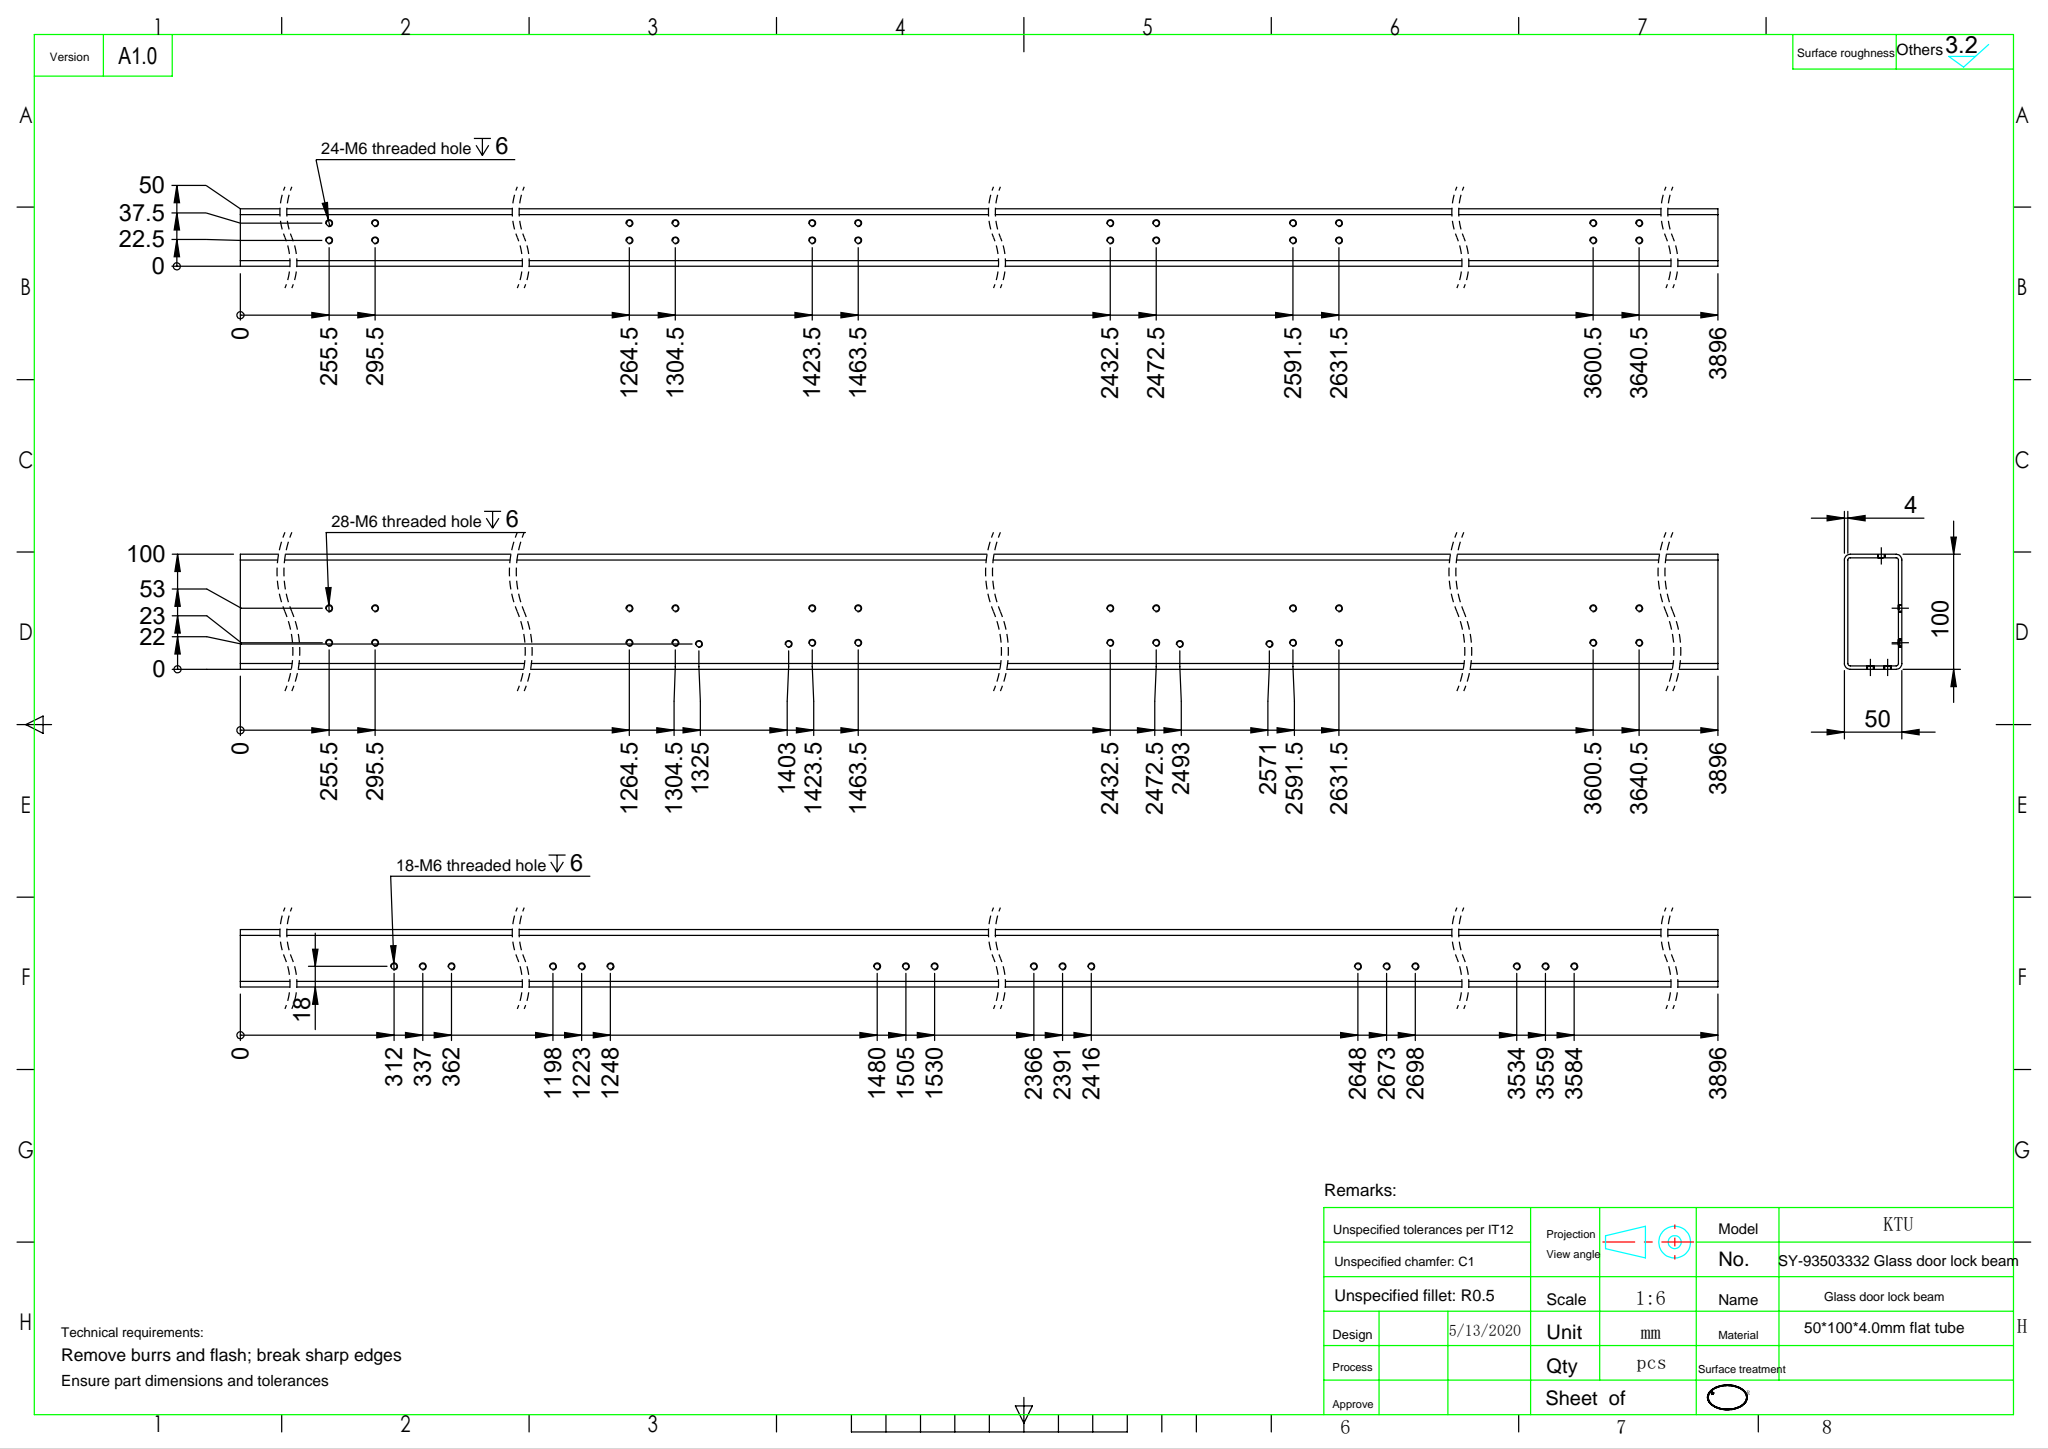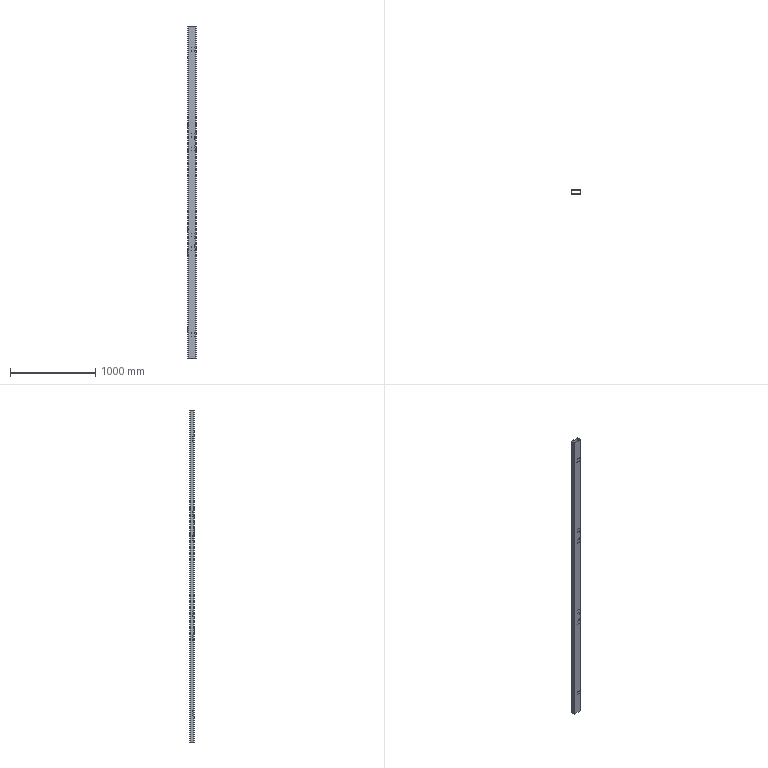Part | SolidWorks | features LPattern 6, HoleWzd 4, 3DProfileFeature 1, DelFace 1, ExtruThin 1 | 1 solid | 158 faces | box 100 x 50 x 3896 mm | volume 3291789 mm3 | cylinder 148 | plane 10 | commonest cylinder face diameters 5 x140 4 x4 10 x4